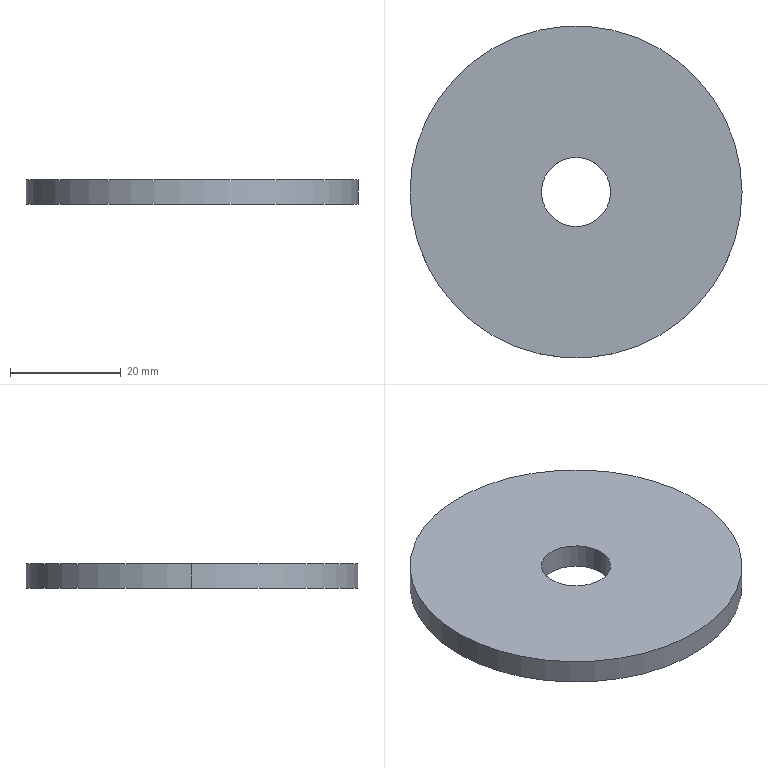Part | STEP file | DCV-000-042 | 1 solid | 6 faces | box 60 x 60 x 4.5 mm | volume 12171 mm3 | cylinder 4 | plane 2 | commonest cylinder face diameters 12.5 x2 60 x2
STEP:
#1=CARTESIAN_POINT('',(0.,0.,0.));
#2=DIRECTION('',(0.,0.,1.));
#3=DIRECTION('',(1.,0.,0.));
#4=AXIS2_PLACEMENT_3D('',#1,#2,#3);
#5=CARTESIAN_POINT('',(6.25,0.,0.));
#6=VERTEX_POINT('',#5);
#7=CARTESIAN_POINT('',(6.25,0.,4.5));
#8=VERTEX_POINT('',#7);
#9=CARTESIAN_POINT('',(6.25,0.,-80.472));
#10=DIRECTION('',(0.,0.,1.));
#11=VECTOR('',#10,1.);
#12=LINE('',#9,#11);
#13=CARTESIAN_POINT('',(0.,0.,-80.472));
#14=DIRECTION('',(0.,0.,1.));
#15=DIRECTION('',(1.,0.,0.));
#16=AXIS2_PLACEMENT_3D('',#13,#14,#15);
#17=CYLINDRICAL_SURFACE('',#16,6.25);
#18=CARTESIAN_POINT('',(6.283,0.));
#19=DIRECTION('',(0.,1.));
#20=VECTOR('',#19,1.);
#21=LINE('',#18,#20);
#22=(GEOMETRIC_REPRESENTATION_CONTEXT(2)PARAMETRIC_REPRESENTATION_CONTEXT()REPRESENTATION_CONTEXT('',''));
#23=DEFINITIONAL_REPRESENTATION('',(#21),#22);
#24=PCURVE('',#17,#23);
#25=CARTESIAN_POINT('',(0.,0.,-80.472));
#26=DIRECTION('',(0.,0.,1.));
#27=DIRECTION('',(1.,0.,0.));
#28=AXIS2_PLACEMENT_3D('',#25,#26,#27);
#29=CYLINDRICAL_SURFACE('',#28,6.25);
#30=CARTESIAN_POINT('',(0.,0.));
#31=DIRECTION('',(0.,1.));
#32=VECTOR('',#31,1.);
#33=LINE('',#30,#32);
#34=(GEOMETRIC_REPRESENTATION_CONTEXT(2)PARAMETRIC_REPRESENTATION_CONTEXT()REPRESENTATION_CONTEXT('',''));
#35=DEFINITIONAL_REPRESENTATION('',(#33),#34);
#36=PCURVE('',#29,#35);
#37=SURFACE_CURVE('',#12,(#24,#36),.PCURVE_S1.);
#38=EDGE_CURVE('',#6,#8,#37,.T.);
#39=ORIENTED_EDGE('',*,*,#38,.T.);
#40=CARTESIAN_POINT('',(-6.25,0.,4.5));
#41=VERTEX_POINT('',#40);
#42=CARTESIAN_POINT('',(0.,0.,4.5));
#43=DIRECTION('',(0.,0.,-1.));
#44=DIRECTION('',(1.,0.,0.));
#45=AXIS2_PLACEMENT_3D('',#42,#43,#44);
#46=CIRCLE('',#45,6.25);
#47=CARTESIAN_POINT('',(6.283,84.972));
#48=DIRECTION('',(-1.,0.));
#49=VECTOR('',#48,1.);
#50=LINE('',#47,#49);
#51=(GEOMETRIC_REPRESENTATION_CONTEXT(2)PARAMETRIC_REPRESENTATION_CONTEXT()REPRESENTATION_CONTEXT('',''));
#52=DEFINITIONAL_REPRESENTATION('',(#50),#51);
#53=PCURVE('',#17,#52);
#54=CARTESIAN_POINT('',(0.,0.,4.5));
#55=DIRECTION('',(0.,0.,1.));
#56=DIRECTION('',(1.,0.,0.));
#57=AXIS2_PLACEMENT_3D('',#54,#55,#56);
#58=PLANE('',#57);
#59=CARTESIAN_POINT('',(6.25,0.));
#60=CARTESIAN_POINT('',(6.25,-10.825));
#61=CARTESIAN_POINT('',(-3.125,-5.413));
#62=CARTESIAN_POINT('',(-12.5,0.));
#63=CARTESIAN_POINT('',(-3.125,5.413));
#64=CARTESIAN_POINT('',(6.25,10.825));
#65=CARTESIAN_POINT('',(6.25,0.));
#66=(BOUNDED_CURVE()B_SPLINE_CURVE(2,(#59,#60,#61,#62,#63,#64,#65),.UNSPECIFIED.,.T.,.F.)B_SPLINE_CURVE_WITH_KNOTS((1,2,2,2,2,1),(-2.094,0.,2.094,4.189,6.283,8.378),.UNSPECIFIED.)CURVE()GEOMETRIC_REPRESENTATION_ITEM()RATIONAL_B_SPLINE_CURVE((1.,0.5,1.,0.5,1.,0.5,1.))REPRESENTATION_ITEM(''));
#67=(GEOMETRIC_REPRESENTATION_CONTEXT(2)PARAMETRIC_REPRESENTATION_CONTEXT()REPRESENTATION_CONTEXT('',''));
#68=DEFINITIONAL_REPRESENTATION('',(#66),#67);
#69=PCURVE('',#58,#68);
#70=SURFACE_CURVE('',#46,(#53,#69),.PCURVE_S1.);
#71=EDGE_CURVE('',#8,#41,#70,.T.);
#72=ORIENTED_EDGE('',*,*,#71,.T.);
#73=CARTESIAN_POINT('',(-6.25,0.,0.));
#74=VERTEX_POINT('',#73);
#75=CARTESIAN_POINT('',(-6.25,0.,-80.472));
#76=DIRECTION('',(0.,0.,1.));
#77=VECTOR('',#76,1.);
#78=LINE('',#75,#77);
#79=CARTESIAN_POINT('',(3.142,0.));
#80=DIRECTION('',(0.,1.));
#81=VECTOR('',#80,1.);
#82=LINE('',#79,#81);
#83=(GEOMETRIC_REPRESENTATION_CONTEXT(2)PARAMETRIC_REPRESENTATION_CONTEXT()REPRESENTATION_CONTEXT('',''));
#84=DEFINITIONAL_REPRESENTATION('',(#82),#83);
#85=PCURVE('',#17,#84);
#86=CARTESIAN_POINT('',(3.142,0.));
#87=DIRECTION('',(0.,1.));
#88=VECTOR('',#87,1.);
#89=LINE('',#86,#88);
#90=(GEOMETRIC_REPRESENTATION_CONTEXT(2)PARAMETRIC_REPRESENTATION_CONTEXT()REPRESENTATION_CONTEXT('',''));
#91=DEFINITIONAL_REPRESENTATION('',(#89),#90);
#92=PCURVE('',#29,#91);
#93=SURFACE_CURVE('',#78,(#85,#92),.PCURVE_S1.);
#94=EDGE_CURVE('',#74,#41,#93,.T.);
#95=ORIENTED_EDGE('',*,*,#94,.F.);
#96=CARTESIAN_POINT('',(0.,0.,0.));
#97=DIRECTION('',(0.,0.,1.));
#98=DIRECTION('',(1.,0.,0.));
#99=AXIS2_PLACEMENT_3D('',#96,#97,#98);
#100=CIRCLE('',#99,6.25);
#101=CARTESIAN_POINT('',(0.,80.472));
#102=DIRECTION('',(1.,0.));
#103=VECTOR('',#102,1.);
#104=LINE('',#101,#103);
#105=(GEOMETRIC_REPRESENTATION_CONTEXT(2)PARAMETRIC_REPRESENTATION_CONTEXT()REPRESENTATION_CONTEXT('',''));
#106=DEFINITIONAL_REPRESENTATION('',(#104),#105);
#107=PCURVE('',#17,#106);
#108=CARTESIAN_POINT('',(0.,0.,0.));
#109=DIRECTION('',(0.,0.,1.));
#110=DIRECTION('',(1.,0.,0.));
#111=AXIS2_PLACEMENT_3D('',#108,#109,#110);
#112=PLANE('',#111);
#113=CARTESIAN_POINT('',(0.,0.));
#114=DIRECTION('',(1.,0.));
#115=AXIS2_PLACEMENT_2D('',#113,#114);
#116=CIRCLE('',#115,6.25);
#117=(GEOMETRIC_REPRESENTATION_CONTEXT(2)PARAMETRIC_REPRESENTATION_CONTEXT()REPRESENTATION_CONTEXT('',''));
#118=DEFINITIONAL_REPRESENTATION('',(#116),#117);
#119=PCURVE('',#112,#118);
#120=SURFACE_CURVE('',#100,(#107,#119),.PCURVE_S1.);
#121=EDGE_CURVE('',#74,#6,#120,.T.);
#122=ORIENTED_EDGE('',*,*,#121,.T.);
#123=EDGE_LOOP('',(#39,#72,#95,#122));
#124=FACE_BOUND('',#123,.F.);
#125=ADVANCED_FACE('',(#124),#17,.F.);
#126=CARTESIAN_POINT('',(30.,0.,0.));
#127=VERTEX_POINT('',#126);
#128=CARTESIAN_POINT('',(-30.,0.,0.));
#129=VERTEX_POINT('',#128);
#130=CARTESIAN_POINT('',(0.,0.,0.));
#131=DIRECTION('',(0.,0.,1.));
#132=DIRECTION('',(1.,0.,0.));
#133=AXIS2_PLACEMENT_3D('',#130,#131,#132);
#134=CIRCLE('',#133,30.);
#135=CARTESIAN_POINT('',(0.,0.,0.));
#136=DIRECTION('',(0.,0.,1.));
#137=DIRECTION('',(1.,0.,0.));
#138=AXIS2_PLACEMENT_3D('',#135,#136,#137);
#139=CYLINDRICAL_SURFACE('',#138,30.);
#140=CARTESIAN_POINT('',(0.,0.));
#141=DIRECTION('',(1.,0.));
#142=VECTOR('',#141,1.);
#143=LINE('',#140,#142);
#144=(GEOMETRIC_REPRESENTATION_CONTEXT(2)PARAMETRIC_REPRESENTATION_CONTEXT()REPRESENTATION_CONTEXT('',''));
#145=DEFINITIONAL_REPRESENTATION('',(#143),#144);
#146=PCURVE('',#139,#145);
#147=CARTESIAN_POINT('',(0.,0.));
#148=DIRECTION('',(1.,0.));
#149=AXIS2_PLACEMENT_2D('',#147,#148);
#150=CIRCLE('',#149,30.);
#151=(GEOMETRIC_REPRESENTATION_CONTEXT(2)PARAMETRIC_REPRESENTATION_CONTEXT()REPRESENTATION_CONTEXT('',''));
#152=DEFINITIONAL_REPRESENTATION('',(#150),#151);
#153=PCURVE('',#112,#152);
#154=SURFACE_CURVE('',#134,(#146,#153),.PCURVE_S1.);
#155=EDGE_CURVE('',#127,#129,#154,.T.);
#156=ORIENTED_EDGE('',*,*,#155,.T.);
#157=CARTESIAN_POINT('',(-30.,0.,4.5));
#158=VERTEX_POINT('',#157);
#159=CARTESIAN_POINT('',(-30.,0.,0.));
#160=DIRECTION('',(0.,0.,1.));
#161=VECTOR('',#160,1.);
#162=LINE('',#159,#161);
#163=CARTESIAN_POINT('',(3.142,0.));
#164=DIRECTION('',(0.,1.));
#165=VECTOR('',#164,1.);
#166=LINE('',#163,#165);
#167=(GEOMETRIC_REPRESENTATION_CONTEXT(2)PARAMETRIC_REPRESENTATION_CONTEXT()REPRESENTATION_CONTEXT('',''));
#168=DEFINITIONAL_REPRESENTATION('',(#166),#167);
#169=PCURVE('',#139,#168);
#170=CARTESIAN_POINT('',(0.,0.,0.));
#171=DIRECTION('',(0.,0.,1.));
#172=DIRECTION('',(1.,0.,0.));
#173=AXIS2_PLACEMENT_3D('',#170,#171,#172);
#174=CYLINDRICAL_SURFACE('',#173,30.);
#175=CARTESIAN_POINT('',(3.142,0.));
#176=DIRECTION('',(0.,1.));
#177=VECTOR('',#176,1.);
#178=LINE('',#175,#177);
#179=(GEOMETRIC_REPRESENTATION_CONTEXT(2)PARAMETRIC_REPRESENTATION_CONTEXT()REPRESENTATION_CONTEXT('',''));
#180=DEFINITIONAL_REPRESENTATION('',(#178),#179);
#181=PCURVE('',#174,#180);
#182=SURFACE_CURVE('',#162,(#169,#181),.PCURVE_S1.);
#183=EDGE_CURVE('',#129,#158,#182,.T.);
#184=ORIENTED_EDGE('',*,*,#183,.T.);
#185=CARTESIAN_POINT('',(30.,0.,4.5));
#186=VERTEX_POINT('',#185);
#187=CARTESIAN_POINT('',(0.,0.,4.5));
#188=DIRECTION('',(0.,0.,1.));
#189=DIRECTION('',(1.,0.,0.));
#190=AXIS2_PLACEMENT_3D('',#187,#188,#189);
#191=CIRCLE('',#190,30.);
#192=CARTESIAN_POINT('',(0.,4.5));
#193=DIRECTION('',(1.,0.));
#194=VECTOR('',#193,1.);
#195=LINE('',#192,#194);
#196=(GEOMETRIC_REPRESENTATION_CONTEXT(2)PARAMETRIC_REPRESENTATION_CONTEXT()REPRESENTATION_CONTEXT('',''));
#197=DEFINITIONAL_REPRESENTATION('',(#195),#196);
#198=PCURVE('',#139,#197);
#199=CARTESIAN_POINT('',(0.,0.));
#200=DIRECTION('',(1.,0.));
#201=AXIS2_PLACEMENT_2D('',#199,#200);
#202=CIRCLE('',#201,30.);
#203=(GEOMETRIC_REPRESENTATION_CONTEXT(2)PARAMETRIC_REPRESENTATION_CONTEXT()REPRESENTATION_CONTEXT('',''));
#204=DEFINITIONAL_REPRESENTATION('',(#202),#203);
#205=PCURVE('',#58,#204);
#206=SURFACE_CURVE('',#191,(#198,#205),.PCURVE_S1.);
#207=EDGE_CURVE('',#186,#158,#206,.T.);
#208=ORIENTED_EDGE('',*,*,#207,.F.);
#209=CARTESIAN_POINT('',(30.,0.,0.));
#210=DIRECTION('',(0.,0.,1.));
#211=VECTOR('',#210,1.);
#212=LINE('',#209,#211);
#213=CARTESIAN_POINT('',(0.,0.));
#214=DIRECTION('',(0.,1.));
#215=VECTOR('',#214,1.);
#216=LINE('',#213,#215);
#217=(GEOMETRIC_REPRESENTATION_CONTEXT(2)PARAMETRIC_REPRESENTATION_CONTEXT()REPRESENTATION_CONTEXT('',''));
#218=DEFINITIONAL_REPRESENTATION('',(#216),#217);
#219=PCURVE('',#139,#218);
#220=CARTESIAN_POINT('',(6.283,0.));
#221=DIRECTION('',(0.,1.));
#222=VECTOR('',#221,1.);
#223=LINE('',#220,#222);
#224=(GEOMETRIC_REPRESENTATION_CONTEXT(2)PARAMETRIC_REPRESENTATION_CONTEXT()REPRESENTATION_CONTEXT('',''));
#225=DEFINITIONAL_REPRESENTATION('',(#223),#224);
#226=PCURVE('',#174,#225);
#227=SURFACE_CURVE('',#212,(#219,#226),.PCURVE_S1.);
#228=EDGE_CURVE('',#127,#186,#227,.T.);
#229=ORIENTED_EDGE('',*,*,#228,.F.);
#230=EDGE_LOOP('',(#156,#184,#208,#229));
#231=FACE_BOUND('',#230,.T.);
#232=ADVANCED_FACE('',(#231),#139,.T.);
#233=CARTESIAN_POINT('',(0.,0.,0.));
#234=DIRECTION('',(0.,0.,1.));
#235=DIRECTION('',(1.,0.,0.));
#236=AXIS2_PLACEMENT_3D('',#233,#234,#235);
#237=CIRCLE('',#236,6.25);
#238=CARTESIAN_POINT('',(0.,0.));
#239=DIRECTION('',(1.,0.));
#240=AXIS2_PLACEMENT_2D('',#238,#239);
#241=CIRCLE('',#240,6.25);
#242=(GEOMETRIC_REPRESENTATION_CONTEXT(2)PARAMETRIC_REPRESENTATION_CONTEXT()REPRESENTATION_CONTEXT('',''));
#243=DEFINITIONAL_REPRESENTATION('',(#241),#242);
#244=PCURVE('',#112,#243);
#245=CARTESIAN_POINT('',(0.,80.472));
#246=DIRECTION('',(1.,0.));
#247=VECTOR('',#246,1.);
#248=LINE('',#245,#247);
#249=(GEOMETRIC_REPRESENTATION_CONTEXT(2)PARAMETRIC_REPRESENTATION_CONTEXT()REPRESENTATION_CONTEXT('',''));
#250=DEFINITIONAL_REPRESENTATION('',(#248),#249);
#251=PCURVE('',#29,#250);
#252=SURFACE_CURVE('',#237,(#244,#251),.PCURVE_S1.);
#253=EDGE_CURVE('',#6,#74,#252,.T.);
#254=ORIENTED_EDGE('',*,*,#253,.T.);
#255=ORIENTED_EDGE('',*,*,#121,.T.);
#256=EDGE_LOOP('',(#254,#255));
#257=FACE_BOUND('',#256,.T.);
#258=ORIENTED_EDGE('',*,*,#155,.F.);
#259=CARTESIAN_POINT('',(0.,0.,0.));
#260=DIRECTION('',(0.,0.,1.));
#261=DIRECTION('',(1.,0.,0.));
#262=AXIS2_PLACEMENT_3D('',#259,#260,#261);
#263=CIRCLE('',#262,30.);
#264=CARTESIAN_POINT('',(0.,0.));
#265=DIRECTION('',(1.,0.));
#266=AXIS2_PLACEMENT_2D('',#264,#265);
#267=CIRCLE('',#266,30.);
#268=(GEOMETRIC_REPRESENTATION_CONTEXT(2)PARAMETRIC_REPRESENTATION_CONTEXT()REPRESENTATION_CONTEXT('',''));
#269=DEFINITIONAL_REPRESENTATION('',(#267),#268);
#270=PCURVE('',#112,#269);
#271=CARTESIAN_POINT('',(0.,0.));
#272=DIRECTION('',(1.,0.));
#273=VECTOR('',#272,1.);
#274=LINE('',#271,#273);
#275=(GEOMETRIC_REPRESENTATION_CONTEXT(2)PARAMETRIC_REPRESENTATION_CONTEXT()REPRESENTATION_CONTEXT('',''));
#276=DEFINITIONAL_REPRESENTATION('',(#274),#275);
#277=PCURVE('',#174,#276);
#278=SURFACE_CURVE('',#263,(#270,#277),.PCURVE_S1.);
#279=EDGE_CURVE('',#129,#127,#278,.T.);
#280=ORIENTED_EDGE('',*,*,#279,.F.);
#281=EDGE_LOOP('',(#258,#280));
#282=FACE_BOUND('',#281,.T.);
#283=ADVANCED_FACE('',(#257,#282),#112,.F.);
#284=ORIENTED_EDGE('',*,*,#71,.T.);
#285=CARTESIAN_POINT('',(0.,0.,4.5));
#286=DIRECTION('',(0.,0.,-1.));
#287=DIRECTION('',(1.,0.,0.));
#288=AXIS2_PLACEMENT_3D('',#285,#286,#287);
#289=CIRCLE('',#288,6.25);
#290=CARTESIAN_POINT('',(6.25,0.));
#291=CARTESIAN_POINT('',(6.25,-10.825));
#292=CARTESIAN_POINT('',(-3.125,-5.413));
#293=CARTESIAN_POINT('',(-12.5,0.));
#294=CARTESIAN_POINT('',(-3.125,5.413));
#295=CARTESIAN_POINT('',(6.25,10.825));
#296=CARTESIAN_POINT('',(6.25,0.));
#297=(BOUNDED_CURVE()B_SPLINE_CURVE(2,(#290,#291,#292,#293,#294,#295,#296),.UNSPECIFIED.,.T.,.F.)B_SPLINE_CURVE_WITH_KNOTS((1,2,2,2,2,1),(-2.094,0.,2.094,4.189,6.283,8.378),.UNSPECIFIED.)CURVE()GEOMETRIC_REPRESENTATION_ITEM()RATIONAL_B_SPLINE_CURVE((1.,0.5,1.,0.5,1.,0.5,1.))REPRESENTATION_ITEM(''));
#298=(GEOMETRIC_REPRESENTATION_CONTEXT(2)PARAMETRIC_REPRESENTATION_CONTEXT()REPRESENTATION_CONTEXT('',''));
#299=DEFINITIONAL_REPRESENTATION('',(#297),#298);
#300=PCURVE('',#58,#299);
#301=CARTESIAN_POINT('',(6.283,84.972));
#302=DIRECTION('',(-1.,0.));
#303=VECTOR('',#302,1.);
#304=LINE('',#301,#303);
#305=(GEOMETRIC_REPRESENTATION_CONTEXT(2)PARAMETRIC_REPRESENTATION_CONTEXT()REPRESENTATION_CONTEXT('',''));
#306=DEFINITIONAL_REPRESENTATION('',(#304),#305);
#307=PCURVE('',#29,#306);
#308=SURFACE_CURVE('',#289,(#300,#307),.PCURVE_S1.);
#309=EDGE_CURVE('',#41,#8,#308,.T.);
#310=ORIENTED_EDGE('',*,*,#309,.T.);
#311=EDGE_LOOP('',(#284,#310));
#312=FACE_BOUND('',#311,.T.);
#313=ORIENTED_EDGE('',*,*,#207,.T.);
#314=CARTESIAN_POINT('',(0.,0.,4.5));
#315=DIRECTION('',(0.,0.,1.));
#316=DIRECTION('',(1.,0.,0.));
#317=AXIS2_PLACEMENT_3D('',#314,#315,#316);
#318=CIRCLE('',#317,30.);
#319=CARTESIAN_POINT('',(0.,0.));
#320=DIRECTION('',(1.,0.));
#321=AXIS2_PLACEMENT_2D('',#319,#320);
#322=CIRCLE('',#321,30.);
#323=(GEOMETRIC_REPRESENTATION_CONTEXT(2)PARAMETRIC_REPRESENTATION_CONTEXT()REPRESENTATION_CONTEXT('',''));
#324=DEFINITIONAL_REPRESENTATION('',(#322),#323);
#325=PCURVE('',#58,#324);
#326=CARTESIAN_POINT('',(0.,4.5));
#327=DIRECTION('',(1.,0.));
#328=VECTOR('',#327,1.);
#329=LINE('',#326,#328);
#330=(GEOMETRIC_REPRESENTATION_CONTEXT(2)PARAMETRIC_REPRESENTATION_CONTEXT()REPRESENTATION_CONTEXT('',''));
#331=DEFINITIONAL_REPRESENTATION('',(#329),#330);
#332=PCURVE('',#174,#331);
#333=SURFACE_CURVE('',#318,(#325,#332),.PCURVE_S1.);
#334=EDGE_CURVE('',#158,#186,#333,.T.);
#335=ORIENTED_EDGE('',*,*,#334,.T.);
#336=EDGE_LOOP('',(#313,#335));
#337=FACE_BOUND('',#336,.T.);
#338=ADVANCED_FACE('',(#312,#337),#58,.T.);
#339=ORIENTED_EDGE('',*,*,#183,.F.);
#340=ORIENTED_EDGE('',*,*,#279,.T.);
#341=ORIENTED_EDGE('',*,*,#228,.T.);
#342=ORIENTED_EDGE('',*,*,#334,.F.);
#343=EDGE_LOOP('',(#339,#340,#341,#342));
#344=FACE_BOUND('',#343,.T.);
#345=ADVANCED_FACE('',(#344),#174,.T.);
#346=ORIENTED_EDGE('',*,*,#309,.T.);
#347=ORIENTED_EDGE('',*,*,#38,.F.);
#348=ORIENTED_EDGE('',*,*,#253,.T.);
#349=ORIENTED_EDGE('',*,*,#94,.T.);
#350=EDGE_LOOP('',(#346,#347,#348,#349));
#351=FACE_BOUND('',#350,.F.);
#352=ADVANCED_FACE('',(#351),#29,.F.);
#353=CLOSED_SHELL('',(#125,#232,#283,#338,#345,#352));
#354=MANIFOLD_SOLID_BREP('',#353);
#355=(LENGTH_UNIT()NAMED_UNIT(*)SI_UNIT(.MILLI.,.METRE.));
#356=UNCERTAINTY_MEASURE_WITH_UNIT(LENGTH_MEASURE(0.0000001),#355,'','');
#357=(NAMED_UNIT(*)PLANE_ANGLE_UNIT()SI_UNIT($,.RADIAN.));
#358=(NAMED_UNIT(*)SI_UNIT($,.STERADIAN.)SOLID_ANGLE_UNIT());
#359=(GEOMETRIC_REPRESENTATION_CONTEXT(3)GLOBAL_UNCERTAINTY_ASSIGNED_CONTEXT((#356))GLOBAL_UNIT_ASSIGNED_CONTEXT((#355,#357,#358))REPRESENTATION_CONTEXT('',''));
#360=ADVANCED_BREP_SHAPE_REPRESENTATION('',(#4,#354),#359);